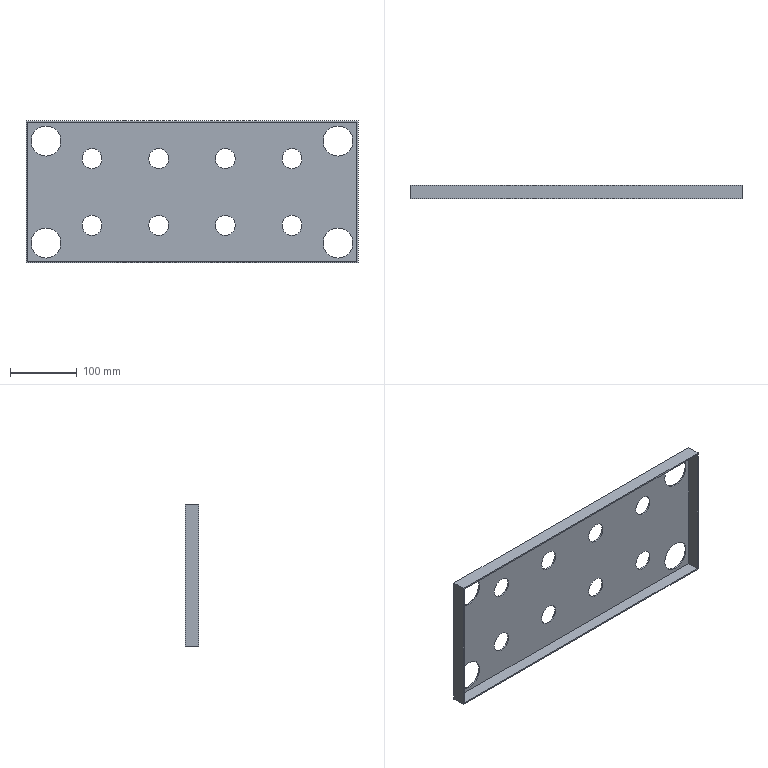Part | NX | 1 solid | 23 faces | box 498 x 20 x 213 mm | volume 239019 mm3 | cylinder 12 | plane 11 | commonest cylinder face diameters 30 x8 45 x4
STEP:
#1=CARTESIAN_POINT('',(-249.,0.,-106.5));
#2=VERTEX_POINT('',#1);
#3=CARTESIAN_POINT('',(249.,0.,-106.5));
#4=VERTEX_POINT('',#3);
#5=CARTESIAN_POINT('',(249.,0.,-106.5));
#6=DIRECTION('',(1.,0.,0.));
#7=VECTOR('',#6,1000.);
#8=LINE('',#5,#7);
#9=EDGE_CURVE('',#2,#4,#8,.T.);
#10=ORIENTED_EDGE('',*,*,#9,.F.);
#11=CARTESIAN_POINT('',(-249.,20.,-106.5));
#12=VERTEX_POINT('',#11);
#13=CARTESIAN_POINT('',(-249.,20.,-106.5));
#14=DIRECTION('',(0.,-1.,0.));
#15=VECTOR('',#14,1000.);
#16=LINE('',#13,#15);
#17=EDGE_CURVE('',#12,#2,#16,.T.);
#18=ORIENTED_EDGE('',*,*,#17,.F.);
#19=CARTESIAN_POINT('',(249.,20.,-106.5));
#20=VERTEX_POINT('',#19);
#21=CARTESIAN_POINT('',(249.,20.,-106.5));
#22=DIRECTION('',(1.,0.,0.));
#23=VECTOR('',#22,1000.);
#24=LINE('',#21,#23);
#25=EDGE_CURVE('',#12,#20,#24,.T.);
#26=ORIENTED_EDGE('',*,*,#25,.T.);
#27=CARTESIAN_POINT('',(249.,20.,-106.5));
#28=DIRECTION('',(0.,-1.,0.));
#29=VECTOR('',#28,1000.);
#30=LINE('',#27,#29);
#31=EDGE_CURVE('',#20,#4,#30,.T.);
#32=ORIENTED_EDGE('',*,*,#31,.T.);
#33=EDGE_LOOP('',(#10,#18,#26,#32));
#34=FACE_BOUND('',#33,.T.);
#35=CARTESIAN_POINT('',(249.,20.,-106.5));
#36=DIRECTION('',(0.,0.,-1.));
#37=DIRECTION('',(-1.,0.,0.));
#38=AXIS2_PLACEMENT_3D('',#35,#36,#37);
#39=PLANE('',#38);
#40=ADVANCED_FACE('',(#34),#39,.T.);
#41=CARTESIAN_POINT('',(-249.,0.,106.5));
#42=VERTEX_POINT('',#41);
#43=CARTESIAN_POINT('',(-249.,0.,106.5));
#44=DIRECTION('',(0.,0.,-1.));
#45=VECTOR('',#44,1000.);
#46=LINE('',#43,#45);
#47=EDGE_CURVE('',#42,#2,#46,.T.);
#48=ORIENTED_EDGE('',*,*,#47,.F.);
#49=CARTESIAN_POINT('',(-249.,20.,106.5));
#50=VERTEX_POINT('',#49);
#51=CARTESIAN_POINT('',(-249.,20.,106.5));
#52=DIRECTION('',(0.,-1.,0.));
#53=VECTOR('',#52,1000.);
#54=LINE('',#51,#53);
#55=EDGE_CURVE('',#50,#42,#54,.T.);
#56=ORIENTED_EDGE('',*,*,#55,.F.);
#57=CARTESIAN_POINT('',(-249.,20.,106.5));
#58=DIRECTION('',(0.,0.,-1.));
#59=VECTOR('',#58,1000.);
#60=LINE('',#57,#59);
#61=EDGE_CURVE('',#50,#12,#60,.T.);
#62=ORIENTED_EDGE('',*,*,#61,.T.);
#63=ORIENTED_EDGE('',*,*,#17,.T.);
#64=EDGE_LOOP('',(#48,#56,#62,#63));
#65=FACE_BOUND('',#64,.T.);
#66=CARTESIAN_POINT('',(-249.,20.,106.5));
#67=DIRECTION('',(-1.,0.,0.));
#68=DIRECTION('',(0.,0.,1.));
#69=AXIS2_PLACEMENT_3D('',#66,#67,#68);
#70=PLANE('',#69);
#71=ADVANCED_FACE('',(#65),#70,.T.);
#72=CARTESIAN_POINT('',(249.,0.,106.5));
#73=VERTEX_POINT('',#72);
#74=CARTESIAN_POINT('',(249.,0.,106.5));
#75=DIRECTION('',(-1.,0.,0.));
#76=VECTOR('',#75,1000.);
#77=LINE('',#74,#76);
#78=EDGE_CURVE('',#73,#42,#77,.T.);
#79=ORIENTED_EDGE('',*,*,#78,.F.);
#80=CARTESIAN_POINT('',(249.,20.,106.5));
#81=VERTEX_POINT('',#80);
#82=CARTESIAN_POINT('',(249.,20.,106.5));
#83=DIRECTION('',(0.,-1.,0.));
#84=VECTOR('',#83,1000.);
#85=LINE('',#82,#84);
#86=EDGE_CURVE('',#81,#73,#85,.T.);
#87=ORIENTED_EDGE('',*,*,#86,.F.);
#88=CARTESIAN_POINT('',(249.,20.,106.5));
#89=DIRECTION('',(-1.,0.,0.));
#90=VECTOR('',#89,1000.);
#91=LINE('',#88,#90);
#92=EDGE_CURVE('',#81,#50,#91,.T.);
#93=ORIENTED_EDGE('',*,*,#92,.T.);
#94=ORIENTED_EDGE('',*,*,#55,.T.);
#95=EDGE_LOOP('',(#79,#87,#93,#94));
#96=FACE_BOUND('',#95,.T.);
#97=CARTESIAN_POINT('',(249.,20.,106.5));
#98=DIRECTION('',(0.,0.,1.));
#99=DIRECTION('',(1.,0.,0.));
#100=AXIS2_PLACEMENT_3D('',#97,#98,#99);
#101=PLANE('',#100);
#102=ADVANCED_FACE('',(#96),#101,.T.);
#103=CARTESIAN_POINT('',(249.,0.,106.5));
#104=DIRECTION('',(0.,0.,1.));
#105=VECTOR('',#104,1000.);
#106=LINE('',#103,#105);
#107=EDGE_CURVE('',#4,#73,#106,.T.);
#108=ORIENTED_EDGE('',*,*,#107,.F.);
#109=ORIENTED_EDGE('',*,*,#31,.F.);
#110=CARTESIAN_POINT('',(249.,20.,106.5));
#111=DIRECTION('',(0.,0.,1.));
#112=VECTOR('',#111,1000.);
#113=LINE('',#110,#112);
#114=EDGE_CURVE('',#20,#81,#113,.T.);
#115=ORIENTED_EDGE('',*,*,#114,.T.);
#116=ORIENTED_EDGE('',*,*,#86,.T.);
#117=EDGE_LOOP('',(#108,#109,#115,#116));
#118=FACE_BOUND('',#117,.T.);
#119=CARTESIAN_POINT('',(249.,20.,106.5));
#120=DIRECTION('',(1.,0.,0.));
#121=DIRECTION('',(0.,0.,-1.));
#122=AXIS2_PLACEMENT_3D('',#119,#120,#121);
#123=PLANE('',#122);
#124=ADVANCED_FACE('',(#118),#123,.T.);
#125=CARTESIAN_POINT('',(-50.,20.,65.));
#126=VERTEX_POINT('',#125);
#127=CARTESIAN_POINT('',(-50.,20.,50.));
#128=DIRECTION('',(0.,1.,0.));
#129=DIRECTION('',(0.,0.,1.));
#130=AXIS2_PLACEMENT_3D('',#127,#128,#129);
#131=CIRCLE('',#130,15.);
#132=EDGE_CURVE('',#126,#126,#131,.T.);
#133=ORIENTED_EDGE('',*,*,#132,.F.);
#134=EDGE_LOOP('',(#133));
#135=FACE_BOUND('',#134,.T.);
#136=CARTESIAN_POINT('',(-150.,20.,65.));
#137=VERTEX_POINT('',#136);
#138=CARTESIAN_POINT('',(-150.,20.,50.));
#139=DIRECTION('',(0.,1.,0.));
#140=DIRECTION('',(0.,0.,1.));
#141=AXIS2_PLACEMENT_3D('',#138,#139,#140);
#142=CIRCLE('',#141,15.);
#143=EDGE_CURVE('',#137,#137,#142,.T.);
#144=ORIENTED_EDGE('',*,*,#143,.F.);
#145=EDGE_LOOP('',(#144));
#146=FACE_BOUND('',#145,.T.);
#147=CARTESIAN_POINT('',(219.,20.,99.));
#148=VERTEX_POINT('',#147);
#149=CARTESIAN_POINT('',(219.,20.,76.5));
#150=DIRECTION('',(0.,1.,0.));
#151=DIRECTION('',(0.,0.,1.));
#152=AXIS2_PLACEMENT_3D('',#149,#150,#151);
#153=CIRCLE('',#152,22.5);
#154=EDGE_CURVE('',#148,#148,#153,.T.);
#155=ORIENTED_EDGE('',*,*,#154,.F.);
#156=EDGE_LOOP('',(#155));
#157=FACE_BOUND('',#156,.T.);
#158=CARTESIAN_POINT('',(219.,20.,-54.));
#159=VERTEX_POINT('',#158);
#160=CARTESIAN_POINT('',(219.,20.,-76.5));
#161=DIRECTION('',(0.,1.,0.));
#162=DIRECTION('',(0.,0.,1.));
#163=AXIS2_PLACEMENT_3D('',#160,#161,#162);
#164=CIRCLE('',#163,22.5);
#165=EDGE_CURVE('',#159,#159,#164,.T.);
#166=ORIENTED_EDGE('',*,*,#165,.F.);
#167=EDGE_LOOP('',(#166));
#168=FACE_BOUND('',#167,.T.);
#169=CARTESIAN_POINT('',(-219.,20.,99.));
#170=VERTEX_POINT('',#169);
#171=CARTESIAN_POINT('',(-219.,20.,76.5));
#172=DIRECTION('',(0.,1.,0.));
#173=DIRECTION('',(0.,0.,1.));
#174=AXIS2_PLACEMENT_3D('',#171,#172,#173);
#175=CIRCLE('',#174,22.5);
#176=EDGE_CURVE('',#170,#170,#175,.T.);
#177=ORIENTED_EDGE('',*,*,#176,.F.);
#178=EDGE_LOOP('',(#177));
#179=FACE_BOUND('',#178,.T.);
#180=CARTESIAN_POINT('',(-219.,20.,-54.));
#181=VERTEX_POINT('',#180);
#182=CARTESIAN_POINT('',(-219.,20.,-76.5));
#183=DIRECTION('',(0.,1.,0.));
#184=DIRECTION('',(0.,0.,1.));
#185=AXIS2_PLACEMENT_3D('',#182,#183,#184);
#186=CIRCLE('',#185,22.5);
#187=EDGE_CURVE('',#181,#181,#186,.T.);
#188=ORIENTED_EDGE('',*,*,#187,.F.);
#189=EDGE_LOOP('',(#188));
#190=FACE_BOUND('',#189,.T.);
#191=ORIENTED_EDGE('',*,*,#25,.F.);
#192=ORIENTED_EDGE('',*,*,#61,.F.);
#193=ORIENTED_EDGE('',*,*,#92,.F.);
#194=ORIENTED_EDGE('',*,*,#114,.F.);
#195=EDGE_LOOP('',(#191,#192,#193,#194));
#196=FACE_BOUND('',#195,.T.);
#197=CARTESIAN_POINT('',(50.,20.,65.));
#198=VERTEX_POINT('',#197);
#199=CARTESIAN_POINT('',(50.,20.,50.));
#200=DIRECTION('',(0.,1.,0.));
#201=DIRECTION('',(0.,0.,1.));
#202=AXIS2_PLACEMENT_3D('',#199,#200,#201);
#203=CIRCLE('',#202,15.);
#204=EDGE_CURVE('',#198,#198,#203,.T.);
#205=ORIENTED_EDGE('',*,*,#204,.F.);
#206=EDGE_LOOP('',(#205));
#207=FACE_BOUND('',#206,.T.);
#208=CARTESIAN_POINT('',(150.,20.,65.));
#209=VERTEX_POINT('',#208);
#210=CARTESIAN_POINT('',(150.,20.,50.));
#211=DIRECTION('',(0.,1.,0.));
#212=DIRECTION('',(0.,0.,1.));
#213=AXIS2_PLACEMENT_3D('',#210,#211,#212);
#214=CIRCLE('',#213,15.);
#215=EDGE_CURVE('',#209,#209,#214,.T.);
#216=ORIENTED_EDGE('',*,*,#215,.F.);
#217=EDGE_LOOP('',(#216));
#218=FACE_BOUND('',#217,.T.);
#219=CARTESIAN_POINT('',(-150.,20.,-35.));
#220=VERTEX_POINT('',#219);
#221=CARTESIAN_POINT('',(-150.,20.,-50.));
#222=DIRECTION('',(0.,1.,0.));
#223=DIRECTION('',(0.,0.,1.));
#224=AXIS2_PLACEMENT_3D('',#221,#222,#223);
#225=CIRCLE('',#224,15.);
#226=EDGE_CURVE('',#220,#220,#225,.T.);
#227=ORIENTED_EDGE('',*,*,#226,.F.);
#228=EDGE_LOOP('',(#227));
#229=FACE_BOUND('',#228,.T.);
#230=CARTESIAN_POINT('',(-50.,20.,-35.));
#231=VERTEX_POINT('',#230);
#232=CARTESIAN_POINT('',(-50.,20.,-50.));
#233=DIRECTION('',(0.,1.,0.));
#234=DIRECTION('',(0.,0.,1.));
#235=AXIS2_PLACEMENT_3D('',#232,#233,#234);
#236=CIRCLE('',#235,15.);
#237=EDGE_CURVE('',#231,#231,#236,.T.);
#238=ORIENTED_EDGE('',*,*,#237,.F.);
#239=EDGE_LOOP('',(#238));
#240=FACE_BOUND('',#239,.T.);
#241=CARTESIAN_POINT('',(50.,20.,-35.));
#242=VERTEX_POINT('',#241);
#243=CARTESIAN_POINT('',(50.,20.,-50.));
#244=DIRECTION('',(0.,1.,0.));
#245=DIRECTION('',(0.,0.,1.));
#246=AXIS2_PLACEMENT_3D('',#243,#244,#245);
#247=CIRCLE('',#246,15.);
#248=EDGE_CURVE('',#242,#242,#247,.T.);
#249=ORIENTED_EDGE('',*,*,#248,.F.);
#250=EDGE_LOOP('',(#249));
#251=FACE_BOUND('',#250,.T.);
#252=CARTESIAN_POINT('',(150.,20.,-35.));
#253=VERTEX_POINT('',#252);
#254=CARTESIAN_POINT('',(150.,20.,-50.));
#255=DIRECTION('',(0.,1.,0.));
#256=DIRECTION('',(0.,0.,1.));
#257=AXIS2_PLACEMENT_3D('',#254,#255,#256);
#258=CIRCLE('',#257,15.);
#259=EDGE_CURVE('',#253,#253,#258,.T.);
#260=ORIENTED_EDGE('',*,*,#259,.F.);
#261=EDGE_LOOP('',(#260));
#262=FACE_BOUND('',#261,.T.);
#263=CARTESIAN_POINT('',(0.,20.,0.));
#264=DIRECTION('',(0.,-1.,0.));
#265=DIRECTION('',(0.,0.,-1.));
#266=AXIS2_PLACEMENT_3D('',#263,#264,#265);
#267=PLANE('',#266);
#268=ADVANCED_FACE('',(#135,#146,#157,#168,#179,#190,#196,#207,#218,#229,#240,#251,#262),#267,.F.);
#269=CARTESIAN_POINT('',(-247.,0.,-104.5));
#270=VERTEX_POINT('',#269);
#271=CARTESIAN_POINT('',(247.,0.,-104.5));
#272=VERTEX_POINT('',#271);
#273=CARTESIAN_POINT('',(0.,0.,-104.5));
#274=DIRECTION('',(1.,0.,0.));
#275=VECTOR('',#274,1000.);
#276=LINE('',#273,#275);
#277=EDGE_CURVE('',#270,#272,#276,.T.);
#278=ORIENTED_EDGE('',*,*,#277,.F.);
#279=CARTESIAN_POINT('',(-247.,0.,104.5));
#280=VERTEX_POINT('',#279);
#281=CARTESIAN_POINT('',(-247.,0.,0.));
#282=DIRECTION('',(0.,0.,-1.));
#283=VECTOR('',#282,1000.);
#284=LINE('',#281,#283);
#285=EDGE_CURVE('',#280,#270,#284,.T.);
#286=ORIENTED_EDGE('',*,*,#285,.F.);
#287=CARTESIAN_POINT('',(247.,0.,104.5));
#288=VERTEX_POINT('',#287);
#289=CARTESIAN_POINT('',(0.,0.,104.5));
#290=DIRECTION('',(-1.,0.,0.));
#291=VECTOR('',#290,1000.);
#292=LINE('',#289,#291);
#293=EDGE_CURVE('',#288,#280,#292,.T.);
#294=ORIENTED_EDGE('',*,*,#293,.F.);
#295=CARTESIAN_POINT('',(247.,0.,0.));
#296=DIRECTION('',(0.,0.,1.));
#297=VECTOR('',#296,1000.);
#298=LINE('',#295,#297);
#299=EDGE_CURVE('',#272,#288,#298,.T.);
#300=ORIENTED_EDGE('',*,*,#299,.F.);
#301=EDGE_LOOP('',(#278,#286,#294,#300));
#302=FACE_BOUND('',#301,.T.);
#303=ORIENTED_EDGE('',*,*,#9,.T.);
#304=ORIENTED_EDGE('',*,*,#107,.T.);
#305=ORIENTED_EDGE('',*,*,#78,.T.);
#306=ORIENTED_EDGE('',*,*,#47,.T.);
#307=EDGE_LOOP('',(#303,#304,#305,#306));
#308=FACE_BOUND('',#307,.T.);
#309=CARTESIAN_POINT('',(0.,0.,0.));
#310=DIRECTION('',(0.,-1.,0.));
#311=DIRECTION('',(0.,0.,-1.));
#312=AXIS2_PLACEMENT_3D('',#309,#310,#311);
#313=PLANE('',#312);
#314=ADVANCED_FACE('',(#302,#308),#313,.T.);
#315=ORIENTED_EDGE('',*,*,#277,.T.);
#316=CARTESIAN_POINT('',(247.,18.,-104.5));
#317=VERTEX_POINT('',#316);
#318=CARTESIAN_POINT('',(247.,20.,-104.5));
#319=DIRECTION('',(0.,-1.,0.));
#320=VECTOR('',#319,1000.);
#321=LINE('',#318,#320);
#322=EDGE_CURVE('',#317,#272,#321,.T.);
#323=ORIENTED_EDGE('',*,*,#322,.F.);
#324=CARTESIAN_POINT('',(-247.,18.,-104.5));
#325=VERTEX_POINT('',#324);
#326=CARTESIAN_POINT('',(0.,18.,-104.5));
#327=DIRECTION('',(1.,0.,0.));
#328=VECTOR('',#327,1000.);
#329=LINE('',#326,#328);
#330=EDGE_CURVE('',#325,#317,#329,.T.);
#331=ORIENTED_EDGE('',*,*,#330,.F.);
#332=CARTESIAN_POINT('',(-247.,20.,-104.5));
#333=DIRECTION('',(0.,-1.,0.));
#334=VECTOR('',#333,1000.);
#335=LINE('',#332,#334);
#336=EDGE_CURVE('',#325,#270,#335,.T.);
#337=ORIENTED_EDGE('',*,*,#336,.T.);
#338=EDGE_LOOP('',(#315,#323,#331,#337));
#339=FACE_BOUND('',#338,.T.);
#340=CARTESIAN_POINT('',(249.,20.,-104.5));
#341=DIRECTION('',(0.,0.,-1.));
#342=DIRECTION('',(-1.,0.,0.));
#343=AXIS2_PLACEMENT_3D('',#340,#341,#342);
#344=PLANE('',#343);
#345=ADVANCED_FACE('',(#339),#344,.F.);
#346=ORIENTED_EDGE('',*,*,#285,.T.);
#347=ORIENTED_EDGE('',*,*,#336,.F.);
#348=CARTESIAN_POINT('',(-247.,18.,104.5));
#349=VERTEX_POINT('',#348);
#350=CARTESIAN_POINT('',(-247.,18.,0.));
#351=DIRECTION('',(0.,0.,-1.));
#352=VECTOR('',#351,1000.);
#353=LINE('',#350,#352);
#354=EDGE_CURVE('',#349,#325,#353,.T.);
#355=ORIENTED_EDGE('',*,*,#354,.F.);
#356=CARTESIAN_POINT('',(-247.,20.,104.5));
#357=DIRECTION('',(0.,-1.,0.));
#358=VECTOR('',#357,1000.);
#359=LINE('',#356,#358);
#360=EDGE_CURVE('',#349,#280,#359,.T.);
#361=ORIENTED_EDGE('',*,*,#360,.T.);
#362=EDGE_LOOP('',(#346,#347,#355,#361));
#363=FACE_BOUND('',#362,.T.);
#364=CARTESIAN_POINT('',(-247.,20.,106.5));
#365=DIRECTION('',(-1.,0.,0.));
#366=DIRECTION('',(0.,0.,1.));
#367=AXIS2_PLACEMENT_3D('',#364,#365,#366);
#368=PLANE('',#367);
#369=ADVANCED_FACE('',(#363),#368,.F.);
#370=ORIENTED_EDGE('',*,*,#293,.T.);
#371=ORIENTED_EDGE('',*,*,#360,.F.);
#372=CARTESIAN_POINT('',(247.,18.,104.5));
#373=VERTEX_POINT('',#372);
#374=CARTESIAN_POINT('',(0.,18.,104.5));
#375=DIRECTION('',(-1.,0.,0.));
#376=VECTOR('',#375,1000.);
#377=LINE('',#374,#376);
#378=EDGE_CURVE('',#373,#349,#377,.T.);
#379=ORIENTED_EDGE('',*,*,#378,.F.);
#380=CARTESIAN_POINT('',(247.,20.,104.5));
#381=DIRECTION('',(0.,-1.,0.));
#382=VECTOR('',#381,1000.);
#383=LINE('',#380,#382);
#384=EDGE_CURVE('',#373,#288,#383,.T.);
#385=ORIENTED_EDGE('',*,*,#384,.T.);
#386=EDGE_LOOP('',(#370,#371,#379,#385));
#387=FACE_BOUND('',#386,.T.);
#388=CARTESIAN_POINT('',(249.,20.,104.5));
#389=DIRECTION('',(0.,0.,1.));
#390=DIRECTION('',(1.,0.,0.));
#391=AXIS2_PLACEMENT_3D('',#388,#389,#390);
#392=PLANE('',#391);
#393=ADVANCED_FACE('',(#387),#392,.F.);
#394=ORIENTED_EDGE('',*,*,#299,.T.);
#395=ORIENTED_EDGE('',*,*,#384,.F.);
#396=CARTESIAN_POINT('',(247.,18.,0.));
#397=DIRECTION('',(0.,0.,1.));
#398=VECTOR('',#397,1000.);
#399=LINE('',#396,#398);
#400=EDGE_CURVE('',#317,#373,#399,.T.);
#401=ORIENTED_EDGE('',*,*,#400,.F.);
#402=ORIENTED_EDGE('',*,*,#322,.T.);
#403=EDGE_LOOP('',(#394,#395,#401,#402));
#404=FACE_BOUND('',#403,.T.);
#405=CARTESIAN_POINT('',(247.,20.,106.5));
#406=DIRECTION('',(1.,0.,0.));
#407=DIRECTION('',(0.,0.,-1.));
#408=AXIS2_PLACEMENT_3D('',#405,#406,#407);
#409=PLANE('',#408);
#410=ADVANCED_FACE('',(#404),#409,.F.);
#411=CARTESIAN_POINT('',(-50.,18.,35.));
#412=VERTEX_POINT('',#411);
#413=CARTESIAN_POINT('',(-50.,18.,50.));
#414=DIRECTION('',(0.,-1.,0.));
#415=DIRECTION('',(0.,0.,-1.));
#416=AXIS2_PLACEMENT_3D('',#413,#414,#415);
#417=CIRCLE('',#416,15.);
#418=EDGE_CURVE('',#412,#412,#417,.T.);
#419=ORIENTED_EDGE('',*,*,#418,.F.);
#420=EDGE_LOOP('',(#419));
#421=FACE_BOUND('',#420,.T.);
#422=CARTESIAN_POINT('',(-150.,18.,35.));
#423=VERTEX_POINT('',#422);
#424=CARTESIAN_POINT('',(-150.,18.,50.));
#425=DIRECTION('',(0.,-1.,0.));
#426=DIRECTION('',(0.,0.,-1.));
#427=AXIS2_PLACEMENT_3D('',#424,#425,#426);
#428=CIRCLE('',#427,15.);
#429=EDGE_CURVE('',#423,#423,#428,.T.);
#430=ORIENTED_EDGE('',*,*,#429,.F.);
#431=EDGE_LOOP('',(#430));
#432=FACE_BOUND('',#431,.T.);
#433=CARTESIAN_POINT('',(219.,18.,54.));
#434=VERTEX_POINT('',#433);
#435=CARTESIAN_POINT('',(219.,18.,76.5));
#436=DIRECTION('',(0.,-1.,0.));
#437=DIRECTION('',(0.,0.,-1.));
#438=AXIS2_PLACEMENT_3D('',#435,#436,#437);
#439=CIRCLE('',#438,22.5);
#440=EDGE_CURVE('',#434,#434,#439,.T.);
#441=ORIENTED_EDGE('',*,*,#440,.F.);
#442=EDGE_LOOP('',(#441));
#443=FACE_BOUND('',#442,.T.);
#444=CARTESIAN_POINT('',(219.,18.,-99.));
#445=VERTEX_POINT('',#444);
#446=CARTESIAN_POINT('',(219.,18.,-76.5));
#447=DIRECTION('',(0.,-1.,0.));
#448=DIRECTION('',(0.,0.,-1.));
#449=AXIS2_PLACEMENT_3D('',#446,#447,#448);
#450=CIRCLE('',#449,22.5);
#451=EDGE_CURVE('',#445,#445,#450,.T.);
#452=ORIENTED_EDGE('',*,*,#451,.F.);
#453=EDGE_LOOP('',(#452));
#454=FACE_BOUND('',#453,.T.);
#455=CARTESIAN_POINT('',(-219.,18.,54.));
#456=VERTEX_POINT('',#455);
#457=CARTESIAN_POINT('',(-219.,18.,76.5));
#458=DIRECTION('',(0.,-1.,0.));
#459=DIRECTION('',(0.,0.,-1.));
#460=AXIS2_PLACEMENT_3D('',#457,#458,#459);
#461=CIRCLE('',#460,22.5);
#462=EDGE_CURVE('',#456,#456,#461,.T.);
#463=ORIENTED_EDGE('',*,*,#462,.F.);
#464=EDGE_LOOP('',(#463));
#465=FACE_BOUND('',#464,.T.);
#466=CARTESIAN_POINT('',(-219.,18.,-99.));
#467=VERTEX_POINT('',#466);
#468=CARTESIAN_POINT('',(-219.,18.,-76.5));
#469=DIRECTION('',(0.,-1.,0.));
#470=DIRECTION('',(0.,0.,-1.));
#471=AXIS2_PLACEMENT_3D('',#468,#469,#470);
#472=CIRCLE('',#471,22.5);
#473=EDGE_CURVE('',#467,#467,#472,.T.);
#474=ORIENTED_EDGE('',*,*,#473,.F.);
#475=EDGE_LOOP('',(#474));
#476=FACE_BOUND('',#475,.T.);
#477=ORIENTED_EDGE('',*,*,#330,.T.);
#478=ORIENTED_EDGE('',*,*,#400,.T.);
#479=ORIENTED_EDGE('',*,*,#378,.T.);
#480=ORIENTED_EDGE('',*,*,#354,.T.);
#481=EDGE_LOOP('',(#477,#478,#479,#480));
#482=FACE_BOUND('',#481,.T.);
#483=CARTESIAN_POINT('',(50.,18.,35.));
#484=VERTEX_POINT('',#483);
#485=CARTESIAN_POINT('',(50.,18.,50.));
#486=DIRECTION('',(0.,-1.,0.));
#487=DIRECTION('',(0.,0.,-1.));
#488=AXIS2_PLACEMENT_3D('',#485,#486,#487);
#489=CIRCLE('',#488,15.);
#490=EDGE_CURVE('',#484,#484,#489,.T.);
#491=ORIENTED_EDGE('',*,*,#490,.F.);
#492=EDGE_LOOP('',(#491));
#493=FACE_BOUND('',#492,.T.);
#494=CARTESIAN_POINT('',(150.,18.,35.));
#495=VERTEX_POINT('',#494);
#496=CARTESIAN_POINT('',(150.,18.,50.));
#497=DIRECTION('',(0.,-1.,0.));
#498=DIRECTION('',(0.,0.,-1.));
#499=AXIS2_PLACEMENT_3D('',#496,#497,#498);
#500=CIRCLE('',#499,15.);
#501=EDGE_CURVE('',#495,#495,#500,.T.);
#502=ORIENTED_EDGE('',*,*,#501,.F.);
#503=EDGE_LOOP('',(#502));
#504=FACE_BOUND('',#503,.T.);
#505=CARTESIAN_POINT('',(-150.,18.,-65.));
#506=VERTEX_POINT('',#505);
#507=CARTESIAN_POINT('',(-150.,18.,-50.));
#508=DIRECTION('',(0.,-1.,0.));
#509=DIRECTION('',(0.,0.,-1.));
#510=AXIS2_PLACEMENT_3D('',#507,#508,#509);
#511=CIRCLE('',#510,15.);
#512=EDGE_CURVE('',#506,#506,#511,.T.);
#513=ORIENTED_EDGE('',*,*,#512,.F.);
#514=EDGE_LOOP('',(#513));
#515=FACE_BOUND('',#514,.T.);
#516=CARTESIAN_POINT('',(-50.,18.,-65.));
#517=VERTEX_POINT('',#516);
#518=CARTESIAN_POINT('',(-50.,18.,-50.));
#519=DIRECTION('',(0.,-1.,0.));
#520=DIRECTION('',(0.,0.,-1.));
#521=AXIS2_PLACEMENT_3D('',#518,#519,#520);
#522=CIRCLE('',#521,15.);
#523=EDGE_CURVE('',#517,#517,#522,.T.);
#524=ORIENTED_EDGE('',*,*,#523,.F.);
#525=EDGE_LOOP('',(#524));
#526=FACE_BOUND('',#525,.T.);
#527=CARTESIAN_POINT('',(50.,18.,-65.));
#528=VERTEX_POINT('',#527);
#529=CARTESIAN_POINT('',(50.,18.,-50.));
#530=DIRECTION('',(0.,-1.,0.));
#531=DIRECTION('',(0.,0.,-1.));
#532=AXIS2_PLACEMENT_3D('',#529,#530,#531);
#533=CIRCLE('',#532,15.);
#534=EDGE_CURVE('',#528,#528,#533,.T.);
#535=ORIENTED_EDGE('',*,*,#534,.F.);
#536=EDGE_LOOP('',(#535));
#537=FACE_BOUND('',#536,.T.);
#538=CARTESIAN_POINT('',(150.,18.,-65.));
#539=VERTEX_POINT('',#538);
#540=CARTESIAN_POINT('',(150.,18.,-50.));
#541=DIRECTION('',(0.,-1.,0.));
#542=DIRECTION('',(0.,0.,-1.));
#543=AXIS2_PLACEMENT_3D('',#540,#541,#542);
#544=CIRCLE('',#543,15.);
#545=EDGE_CURVE('',#539,#539,#544,.T.);
#546=ORIENTED_EDGE('',*,*,#545,.F.);
#547=EDGE_LOOP('',(#546));
#548=FACE_BOUND('',#547,.T.);
#549=CARTESIAN_POINT('',(0.,18.,0.));
#550=DIRECTION('',(0.,-1.,0.));
#551=DIRECTION('',(0.,0.,-1.));
#552=AXIS2_PLACEMENT_3D('',#549,#550,#551);
#553=PLANE('',#552);
#554=ADVANCED_FACE('',(#421,#432,#443,#454,#465,#476,#482,#493,#504,#515,#526,#537,#548),#553,.T.);
#555=ORIENTED_EDGE('',*,*,#473,.T.);
#556=EDGE_LOOP('',(#555));
#557=FACE_BOUND('',#556,.T.);
#558=ORIENTED_EDGE('',*,*,#187,.T.);
#559=EDGE_LOOP('',(#558));
#560=FACE_BOUND('',#559,.T.);
#561=CARTESIAN_POINT('',(-219.,0.,-76.5));
#562=DIRECTION('',(0.,1.,0.));
#563=DIRECTION('',(0.,0.,1.));
#564=AXIS2_PLACEMENT_3D('',#561,#562,#563);
#565=CYLINDRICAL_SURFACE('',#564,22.5);
#566=ADVANCED_FACE('',(#557,#560),#565,.F.);
#567=ORIENTED_EDGE('',*,*,#462,.T.);
#568=EDGE_LOOP('',(#567));
#569=FACE_BOUND('',#568,.T.);
#570=ORIENTED_EDGE('',*,*,#176,.T.);
#571=EDGE_LOOP('',(#570));
#572=FACE_BOUND('',#571,.T.);
#573=CARTESIAN_POINT('',(-219.,0.,76.5));
#574=DIRECTION('',(0.,1.,0.));
#575=DIRECTION('',(0.,0.,1.));
#576=AXIS2_PLACEMENT_3D('',#573,#574,#575);
#577=CYLINDRICAL_SURFACE('',#576,22.5);
#578=ADVANCED_FACE('',(#569,#572),#577,.F.);
#579=ORIENTED_EDGE('',*,*,#451,.T.);
#580=EDGE_LOOP('',(#579));
#581=FACE_BOUND('',#580,.T.);
#582=ORIENTED_EDGE('',*,*,#165,.T.);
#583=EDGE_LOOP('',(#582));
#584=FACE_BOUND('',#583,.T.);
#585=CARTESIAN_POINT('',(219.,0.,-76.5));
#586=DIRECTION('',(0.,1.,0.));
#587=DIRECTION('',(0.,0.,1.));
#588=AXIS2_PLACEMENT_3D('',#585,#586,#587);
#589=CYLINDRICAL_SURFACE('',#588,22.5);
#590=ADVANCED_FACE('',(#581,#584),#589,.F.);
#591=ORIENTED_EDGE('',*,*,#440,.T.);
#592=EDGE_LOOP('',(#591));
#593=FACE_BOUND('',#592,.T.);
#594=ORIENTED_EDGE('',*,*,#154,.T.);
#595=EDGE_LOOP('',(#594));
#596=FACE_BOUND('',#595,.T.);
#597=CARTESIAN_POINT('',(219.,0.,76.5));
#598=DIRECTION('',(0.,1.,0.));
#599=DIRECTION('',(0.,0.,1.));
#600=AXIS2_PLACEMENT_3D('',#597,#598,#599);
#601=CYLINDRICAL_SURFACE('',#600,22.5);
#602=ADVANCED_FACE('',(#593,#596),#601,.F.);
#603=ORIENTED_EDGE('',*,*,#429,.T.);
#604=EDGE_LOOP('',(#603));
#605=FACE_BOUND('',#604,.T.);
#606=ORIENTED_EDGE('',*,*,#143,.T.);
#607=EDGE_LOOP('',(#606));
#608=FACE_BOUND('',#607,.T.);
#609=CARTESIAN_POINT('',(-150.,0.,50.));
#610=DIRECTION('',(0.,1.,0.));
#611=DIRECTION('',(0.,0.,1.));
#612=AXIS2_PLACEMENT_3D('',#609,#610,#611);
#613=CYLINDRICAL_SURFACE('',#612,15.);
#614=ADVANCED_FACE('',(#605,#608),#613,.F.);
#615=ORIENTED_EDGE('',*,*,#418,.T.);
#616=EDGE_LOOP('',(#615));
#617=FACE_BOUND('',#616,.T.);
#618=ORIENTED_EDGE('',*,*,#132,.T.);
#619=EDGE_LOOP('',(#618));
#620=FACE_BOUND('',#619,.T.);
#621=CARTESIAN_POINT('',(-50.,0.,50.));
#622=DIRECTION('',(0.,1.,0.));
#623=DIRECTION('',(0.,0.,1.));
#624=AXIS2_PLACEMENT_3D('',#621,#622,#623);
#625=CYLINDRICAL_SURFACE('',#624,15.);
#626=ADVANCED_FACE('',(#617,#620),#625,.F.);
#627=ORIENTED_EDGE('',*,*,#490,.T.);
#628=EDGE_LOOP('',(#627));
#629=FACE_BOUND('',#628,.T.);
#630=ORIENTED_EDGE('',*,*,#204,.T.);
#631=EDGE_LOOP('',(#630));
#632=FACE_BOUND('',#631,.T.);
#633=CARTESIAN_POINT('',(50.,0.,50.));
#634=DIRECTION('',(0.,1.,0.));
#635=DIRECTION('',(0.,0.,1.));
#636=AXIS2_PLACEMENT_3D('',#633,#634,#635);
#637=CYLINDRICAL_SURFACE('',#636,15.);
#638=ADVANCED_FACE('',(#629,#632),#637,.F.);
#639=ORIENTED_EDGE('',*,*,#501,.T.);
#640=EDGE_LOOP('',(#639));
#641=FACE_BOUND('',#640,.T.);
#642=ORIENTED_EDGE('',*,*,#215,.T.);
#643=EDGE_LOOP('',(#642));
#644=FACE_BOUND('',#643,.T.);
#645=CARTESIAN_POINT('',(150.,0.,50.));
#646=DIRECTION('',(0.,1.,0.));
#647=DIRECTION('',(0.,0.,1.));
#648=AXIS2_PLACEMENT_3D('',#645,#646,#647);
#649=CYLINDRICAL_SURFACE('',#648,15.);
#650=ADVANCED_FACE('',(#641,#644),#649,.F.);
#651=ORIENTED_EDGE('',*,*,#512,.T.);
#652=EDGE_LOOP('',(#651));
#653=FACE_BOUND('',#652,.T.);
#654=ORIENTED_EDGE('',*,*,#226,.T.);
#655=EDGE_LOOP('',(#654));
#656=FACE_BOUND('',#655,.T.);
#657=CARTESIAN_POINT('',(-150.,0.,-50.));
#658=DIRECTION('',(0.,1.,0.));
#659=DIRECTION('',(0.,0.,1.));
#660=AXIS2_PLACEMENT_3D('',#657,#658,#659);
#661=CYLINDRICAL_SURFACE('',#660,15.);
#662=ADVANCED_FACE('',(#653,#656),#661,.F.);
#663=ORIENTED_EDGE('',*,*,#523,.T.);
#664=EDGE_LOOP('',(#663));
#665=FACE_BOUND('',#664,.T.);
#666=ORIENTED_EDGE('',*,*,#237,.T.);
#667=EDGE_LOOP('',(#666));
#668=FACE_BOUND('',#667,.T.);
#669=CARTESIAN_POINT('',(-50.,0.,-50.));
#670=DIRECTION('',(0.,1.,0.));
#671=DIRECTION('',(0.,0.,1.));
#672=AXIS2_PLACEMENT_3D('',#669,#670,#671);
#673=CYLINDRICAL_SURFACE('',#672,15.);
#674=ADVANCED_FACE('',(#665,#668),#673,.F.);
#675=ORIENTED_EDGE('',*,*,#534,.T.);
#676=EDGE_LOOP('',(#675));
#677=FACE_BOUND('',#676,.T.);
#678=ORIENTED_EDGE('',*,*,#248,.T.);
#679=EDGE_LOOP('',(#678));
#680=FACE_BOUND('',#679,.T.);
#681=CARTESIAN_POINT('',(50.,0.,-50.));
#682=DIRECTION('',(0.,1.,0.));
#683=DIRECTION('',(0.,0.,1.));
#684=AXIS2_PLACEMENT_3D('',#681,#682,#683);
#685=CYLINDRICAL_SURFACE('',#684,15.);
#686=ADVANCED_FACE('',(#677,#680),#685,.F.);
#687=ORIENTED_EDGE('',*,*,#545,.T.);
#688=EDGE_LOOP('',(#687));
#689=FACE_BOUND('',#688,.T.);
#690=ORIENTED_EDGE('',*,*,#259,.T.);
#691=EDGE_LOOP('',(#690));
#692=FACE_BOUND('',#691,.T.);
#693=CARTESIAN_POINT('',(150.,0.,-50.));
#694=DIRECTION('',(0.,1.,0.));
#695=DIRECTION('',(0.,0.,1.));
#696=AXIS2_PLACEMENT_3D('',#693,#694,#695);
#697=CYLINDRICAL_SURFACE('',#696,15.);
#698=ADVANCED_FACE('',(#689,#692),#697,.F.);
#699=CLOSED_SHELL('',(#40,#71,#102,#124,#268,#314,#345,#369,#393,#410,#554,#566,#578,#590,#602,#614,#626,#638,#650,#662,#674,#686,#698));
#700=MANIFOLD_SOLID_BREP('',#699);
#701=(LENGTH_UNIT()NAMED_UNIT(*)SI_UNIT(.MILLI.,.METRE.));
#702=UNCERTAINTY_MEASURE_WITH_UNIT(LENGTH_MEASURE(0.00001),#701,'','');
#703=(NAMED_UNIT(*)PLANE_ANGLE_UNIT()SI_UNIT($,.RADIAN.));
#704=(NAMED_UNIT(*)SI_UNIT($,.STERADIAN.)SOLID_ANGLE_UNIT());
#705=(GEOMETRIC_REPRESENTATION_CONTEXT(3)GLOBAL_UNCERTAINTY_ASSIGNED_CONTEXT((#702))GLOBAL_UNIT_ASSIGNED_CONTEXT((#701,#703,#704))REPRESENTATION_CONTEXT('',''));
#706=ADVANCED_BREP_SHAPE_REPRESENTATION('',(#700),#705);